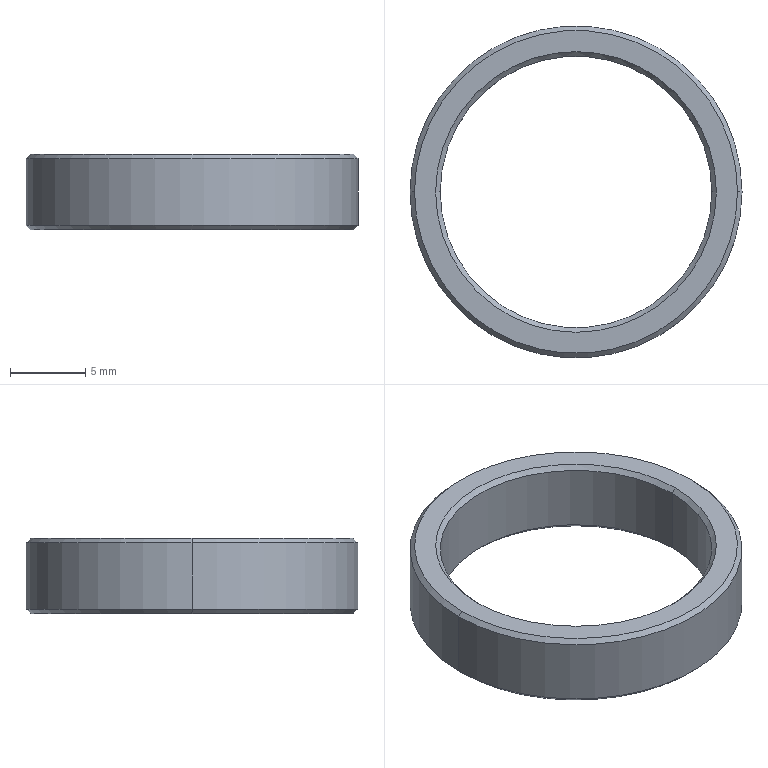Part | SolidWorks | features Chamfer 1, Extrusion 1, ICE 1 | 1 solid | 14 faces | box 22 x 22 x 5 mm | volume 617.009 mm3 | cone 8 | cylinder 4 | plane 2 | commonest cylinder face diameters 18 x2 22 x2
STEP:
#1=CARTESIAN_POINT('',(-9.,0.,4.7));
#2=VERTEX_POINT('',#1);
#3=CARTESIAN_POINT('',(9.,0.,4.7));
#4=VERTEX_POINT('',#3);
#5=CARTESIAN_POINT('',(0.,0.,4.7));
#6=DIRECTION('',(0.,0.,1.));
#7=DIRECTION('',(1.,0.,0.));
#8=AXIS2_PLACEMENT_3D('',#5,#6,#7);
#9=CIRCLE('',#8,9.);
#10=EDGE_CURVE('',#2,#4,#9,.T.);
#11=ORIENTED_EDGE('',*,*,#10,.F.);
#12=CARTESIAN_POINT('',(-9.3,0.,5.));
#13=VERTEX_POINT('',#12);
#14=CARTESIAN_POINT('',(-9.,0.,4.7));
#15=DIRECTION('',(-0.7071,0.,0.7071));
#16=VECTOR('',#15,1000.);
#17=LINE('',#14,#16);
#18=EDGE_CURVE('',#2,#13,#17,.T.);
#19=ORIENTED_EDGE('',*,*,#18,.T.);
#20=CARTESIAN_POINT('',(9.3,0.,5.));
#21=VERTEX_POINT('',#20);
#22=CARTESIAN_POINT('',(0.,0.,5.));
#23=DIRECTION('',(0.,0.,-1.));
#24=DIRECTION('',(1.,0.,0.));
#25=AXIS2_PLACEMENT_3D('',#22,#23,#24);
#26=CIRCLE('',#25,9.3);
#27=EDGE_CURVE('',#21,#13,#26,.T.);
#28=ORIENTED_EDGE('',*,*,#27,.F.);
#29=CARTESIAN_POINT('',(9.,0.,4.7));
#30=DIRECTION('',(0.7071,0.,0.7071));
#31=VECTOR('',#30,1000.);
#32=LINE('',#29,#31);
#33=EDGE_CURVE('',#4,#21,#32,.T.);
#34=ORIENTED_EDGE('',*,*,#33,.F.);
#35=EDGE_LOOP('',(#11,#19,#28,#34));
#36=FACE_OUTER_BOUND('',#35,.T.);
#37=CARTESIAN_POINT('',(0.,0.,4.7));
#38=DIRECTION('',(0.,0.,1.));
#39=DIRECTION('',(1.,0.,0.));
#40=AXIS2_PLACEMENT_3D('',#37,#38,#39);
#41=CONICAL_SURFACE('',#40,9.,0.7854);
#42=ADVANCED_FACE('',(#36),#41,.F.);
#43=CARTESIAN_POINT('',(9.,0.,0.3));
#44=VERTEX_POINT('',#43);
#45=CARTESIAN_POINT('',(-9.,0.,0.3));
#46=VERTEX_POINT('',#45);
#47=CARTESIAN_POINT('',(0.,0.,0.3));
#48=DIRECTION('',(0.,0.,-1.));
#49=DIRECTION('',(1.,0.,0.));
#50=AXIS2_PLACEMENT_3D('',#47,#48,#49);
#51=CIRCLE('',#50,9.);
#52=EDGE_CURVE('',#44,#46,#51,.T.);
#53=ORIENTED_EDGE('',*,*,#52,.F.);
#54=CARTESIAN_POINT('',(9.3,0.,0.));
#55=VERTEX_POINT('',#54);
#56=CARTESIAN_POINT('',(9.3,0.,0.));
#57=DIRECTION('',(0.7071,0.,-0.7071));
#58=VECTOR('',#57,1000.);
#59=LINE('',#56,#58);
#60=EDGE_CURVE('',#44,#55,#59,.T.);
#61=ORIENTED_EDGE('',*,*,#60,.T.);
#62=CARTESIAN_POINT('',(-9.3,0.,0.));
#63=VERTEX_POINT('',#62);
#64=CARTESIAN_POINT('',(0.,0.,0.));
#65=DIRECTION('',(0.,0.,1.));
#66=DIRECTION('',(1.,0.,0.));
#67=AXIS2_PLACEMENT_3D('',#64,#65,#66);
#68=CIRCLE('',#67,9.3);
#69=EDGE_CURVE('',#63,#55,#68,.T.);
#70=ORIENTED_EDGE('',*,*,#69,.F.);
#71=CARTESIAN_POINT('',(-9.3,0.,0.));
#72=DIRECTION('',(-0.7071,0.,-0.7071));
#73=VECTOR('',#72,1000.);
#74=LINE('',#71,#73);
#75=EDGE_CURVE('',#46,#63,#74,.T.);
#76=ORIENTED_EDGE('',*,*,#75,.F.);
#77=EDGE_LOOP('',(#53,#61,#70,#76));
#78=FACE_OUTER_BOUND('',#77,.T.);
#79=CARTESIAN_POINT('',(0.,0.,0.));
#80=DIRECTION('',(0.,0.,-1.));
#81=DIRECTION('',(-1.,0.,0.));
#82=AXIS2_PLACEMENT_3D('',#79,#80,#81);
#83=CONICAL_SURFACE('',#82,9.3,0.7854);
#84=ADVANCED_FACE('',(#78),#83,.F.);
#85=CARTESIAN_POINT('',(10.7,0.,5.));
#86=VERTEX_POINT('',#85);
#87=CARTESIAN_POINT('',(-10.7,0.,5.));
#88=VERTEX_POINT('',#87);
#89=CARTESIAN_POINT('',(0.,0.,5.));
#90=DIRECTION('',(0.,0.,1.));
#91=DIRECTION('',(1.,0.,0.));
#92=AXIS2_PLACEMENT_3D('',#89,#90,#91);
#93=CIRCLE('',#92,10.7);
#94=EDGE_CURVE('',#86,#88,#93,.T.);
#95=ORIENTED_EDGE('',*,*,#94,.F.);
#96=CARTESIAN_POINT('',(11.,0.,4.7));
#97=VERTEX_POINT('',#96);
#98=CARTESIAN_POINT('',(10.7,0.,5.));
#99=DIRECTION('',(0.7071,0.,-0.7071));
#100=VECTOR('',#99,1000.);
#101=LINE('',#98,#100);
#102=EDGE_CURVE('',#86,#97,#101,.T.);
#103=ORIENTED_EDGE('',*,*,#102,.T.);
#104=CARTESIAN_POINT('',(-11.,0.,4.7));
#105=VERTEX_POINT('',#104);
#106=CARTESIAN_POINT('',(0.,0.,4.7));
#107=DIRECTION('',(0.,0.,-1.));
#108=DIRECTION('',(1.,0.,0.));
#109=AXIS2_PLACEMENT_3D('',#106,#107,#108);
#110=CIRCLE('',#109,11.);
#111=EDGE_CURVE('',#105,#97,#110,.T.);
#112=ORIENTED_EDGE('',*,*,#111,.F.);
#113=CARTESIAN_POINT('',(-10.7,0.,5.));
#114=DIRECTION('',(-0.7071,0.,-0.7071));
#115=VECTOR('',#114,1000.);
#116=LINE('',#113,#115);
#117=EDGE_CURVE('',#88,#105,#116,.T.);
#118=ORIENTED_EDGE('',*,*,#117,.F.);
#119=EDGE_LOOP('',(#95,#103,#112,#118));
#120=FACE_OUTER_BOUND('',#119,.T.);
#121=CARTESIAN_POINT('',(0.,0.,5.));
#122=DIRECTION('',(0.,0.,-1.));
#123=DIRECTION('',(-1.,0.,0.));
#124=AXIS2_PLACEMENT_3D('',#121,#122,#123);
#125=CONICAL_SURFACE('',#124,10.7,0.7854);
#126=ADVANCED_FACE('',(#120),#125,.T.);
#127=CARTESIAN_POINT('',(-10.7,0.,0.));
#128=VERTEX_POINT('',#127);
#129=CARTESIAN_POINT('',(10.7,0.,0.));
#130=VERTEX_POINT('',#129);
#131=CARTESIAN_POINT('',(0.,0.,0.));
#132=DIRECTION('',(0.,0.,-1.));
#133=DIRECTION('',(1.,0.,0.));
#134=AXIS2_PLACEMENT_3D('',#131,#132,#133);
#135=CIRCLE('',#134,10.7);
#136=EDGE_CURVE('',#128,#130,#135,.T.);
#137=ORIENTED_EDGE('',*,*,#136,.F.);
#138=CARTESIAN_POINT('',(-11.,0.,0.3));
#139=VERTEX_POINT('',#138);
#140=CARTESIAN_POINT('',(-11.,0.,0.3));
#141=DIRECTION('',(-0.7071,0.,0.7071));
#142=VECTOR('',#141,1000.);
#143=LINE('',#140,#142);
#144=EDGE_CURVE('',#128,#139,#143,.T.);
#145=ORIENTED_EDGE('',*,*,#144,.T.);
#146=CARTESIAN_POINT('',(11.,0.,0.3));
#147=VERTEX_POINT('',#146);
#148=CARTESIAN_POINT('',(0.,0.,0.3));
#149=DIRECTION('',(0.,0.,1.));
#150=DIRECTION('',(1.,0.,0.));
#151=AXIS2_PLACEMENT_3D('',#148,#149,#150);
#152=CIRCLE('',#151,11.);
#153=EDGE_CURVE('',#147,#139,#152,.T.);
#154=ORIENTED_EDGE('',*,*,#153,.F.);
#155=CARTESIAN_POINT('',(11.,0.,0.3));
#156=DIRECTION('',(0.7071,0.,0.7071));
#157=VECTOR('',#156,1000.);
#158=LINE('',#155,#157);
#159=EDGE_CURVE('',#130,#147,#158,.T.);
#160=ORIENTED_EDGE('',*,*,#159,.F.);
#161=EDGE_LOOP('',(#137,#145,#154,#160));
#162=FACE_OUTER_BOUND('',#161,.T.);
#163=CARTESIAN_POINT('',(0.,0.,0.3));
#164=DIRECTION('',(0.,0.,1.));
#165=DIRECTION('',(1.,0.,0.));
#166=AXIS2_PLACEMENT_3D('',#163,#164,#165);
#167=CONICAL_SURFACE('',#166,11.,0.7854);
#168=ADVANCED_FACE('',(#162),#167,.T.);
#169=ORIENTED_EDGE('',*,*,#52,.T.);
#170=CARTESIAN_POINT('',(-9.,0.,0.));
#171=DIRECTION('',(0.,0.,1.));
#172=VECTOR('',#171,1000.);
#173=LINE('',#170,#172);
#174=EDGE_CURVE('',#46,#2,#173,.T.);
#175=ORIENTED_EDGE('',*,*,#174,.T.);
#176=ORIENTED_EDGE('',*,*,#10,.T.);
#177=CARTESIAN_POINT('',(9.,0.,0.));
#178=DIRECTION('',(0.,0.,1.));
#179=VECTOR('',#178,1000.);
#180=LINE('',#177,#179);
#181=EDGE_CURVE('',#44,#4,#180,.T.);
#182=ORIENTED_EDGE('',*,*,#181,.F.);
#183=EDGE_LOOP('',(#169,#175,#176,#182));
#184=FACE_OUTER_BOUND('',#183,.T.);
#185=CARTESIAN_POINT('',(0.,0.,0.));
#186=DIRECTION('',(0.,0.,1.));
#187=DIRECTION('',(1.,0.,0.));
#188=AXIS2_PLACEMENT_3D('',#185,#186,#187);
#189=CYLINDRICAL_SURFACE('',#188,9.);
#190=ADVANCED_FACE('',(#184),#189,.F.);
#191=ORIENTED_EDGE('',*,*,#111,.T.);
#192=CARTESIAN_POINT('',(11.,0.,5.));
#193=DIRECTION('',(0.,0.,-1.));
#194=VECTOR('',#193,1000.);
#195=LINE('',#192,#194);
#196=EDGE_CURVE('',#97,#147,#195,.T.);
#197=ORIENTED_EDGE('',*,*,#196,.T.);
#198=ORIENTED_EDGE('',*,*,#153,.T.);
#199=CARTESIAN_POINT('',(-11.,0.,5.));
#200=DIRECTION('',(0.,0.,-1.));
#201=VECTOR('',#200,1000.);
#202=LINE('',#199,#201);
#203=EDGE_CURVE('',#105,#139,#202,.T.);
#204=ORIENTED_EDGE('',*,*,#203,.F.);
#205=EDGE_LOOP('',(#191,#197,#198,#204));
#206=FACE_OUTER_BOUND('',#205,.T.);
#207=CARTESIAN_POINT('',(0.,0.,5.));
#208=DIRECTION('',(0.,0.,-1.));
#209=DIRECTION('',(-1.,0.,0.));
#210=AXIS2_PLACEMENT_3D('',#207,#208,#209);
#211=CYLINDRICAL_SURFACE('',#210,11.);
#212=ADVANCED_FACE('',(#206),#211,.T.);
#213=ORIENTED_EDGE('',*,*,#196,.F.);
#214=CARTESIAN_POINT('',(0.,0.,4.7));
#215=DIRECTION('',(0.,0.,-1.));
#216=DIRECTION('',(1.,0.,0.));
#217=AXIS2_PLACEMENT_3D('',#214,#215,#216);
#218=CIRCLE('',#217,11.);
#219=EDGE_CURVE('',#97,#105,#218,.T.);
#220=ORIENTED_EDGE('',*,*,#219,.T.);
#221=ORIENTED_EDGE('',*,*,#203,.T.);
#222=CARTESIAN_POINT('',(0.,0.,0.3));
#223=DIRECTION('',(0.,0.,1.));
#224=DIRECTION('',(1.,0.,0.));
#225=AXIS2_PLACEMENT_3D('',#222,#223,#224);
#226=CIRCLE('',#225,11.);
#227=EDGE_CURVE('',#139,#147,#226,.T.);
#228=ORIENTED_EDGE('',*,*,#227,.T.);
#229=EDGE_LOOP('',(#213,#220,#221,#228));
#230=FACE_OUTER_BOUND('',#229,.T.);
#231=CARTESIAN_POINT('',(0.,0.,5.));
#232=DIRECTION('',(0.,0.,-1.));
#233=DIRECTION('',(-1.,0.,0.));
#234=AXIS2_PLACEMENT_3D('',#231,#232,#233);
#235=CYLINDRICAL_SURFACE('',#234,11.);
#236=ADVANCED_FACE('',(#230),#235,.T.);
#237=CARTESIAN_POINT('',(0.,0.,5.));
#238=DIRECTION('',(0.,0.,1.));
#239=DIRECTION('',(1.,0.,0.));
#240=AXIS2_PLACEMENT_3D('',#237,#238,#239);
#241=CIRCLE('',#240,10.7);
#242=EDGE_CURVE('',#88,#86,#241,.T.);
#243=ORIENTED_EDGE('',*,*,#242,.T.);
#244=ORIENTED_EDGE('',*,*,#94,.T.);
#245=EDGE_LOOP('',(#243,#244));
#246=FACE_OUTER_BOUND('',#245,.T.);
#247=ORIENTED_EDGE('',*,*,#27,.T.);
#248=CARTESIAN_POINT('',(0.,0.,5.));
#249=DIRECTION('',(0.,0.,-1.));
#250=DIRECTION('',(1.,0.,0.));
#251=AXIS2_PLACEMENT_3D('',#248,#249,#250);
#252=CIRCLE('',#251,9.3);
#253=EDGE_CURVE('',#13,#21,#252,.T.);
#254=ORIENTED_EDGE('',*,*,#253,.T.);
#255=EDGE_LOOP('',(#247,#254));
#256=FACE_BOUND('',#255,.T.);
#257=CARTESIAN_POINT('',(0.,0.,5.));
#258=DIRECTION('',(0.,0.,1.));
#259=DIRECTION('',(1.,0.,0.));
#260=AXIS2_PLACEMENT_3D('',#257,#258,#259);
#261=PLANE('',#260);
#262=ADVANCED_FACE('',(#246,#256),#261,.T.);
#263=CARTESIAN_POINT('',(0.,0.,0.));
#264=DIRECTION('',(0.,0.,-1.));
#265=DIRECTION('',(1.,0.,0.));
#266=AXIS2_PLACEMENT_3D('',#263,#264,#265);
#267=CIRCLE('',#266,10.7);
#268=EDGE_CURVE('',#130,#128,#267,.T.);
#269=ORIENTED_EDGE('',*,*,#268,.T.);
#270=ORIENTED_EDGE('',*,*,#136,.T.);
#271=EDGE_LOOP('',(#269,#270));
#272=FACE_OUTER_BOUND('',#271,.T.);
#273=ORIENTED_EDGE('',*,*,#69,.T.);
#274=CARTESIAN_POINT('',(0.,0.,0.));
#275=DIRECTION('',(0.,0.,1.));
#276=DIRECTION('',(1.,0.,0.));
#277=AXIS2_PLACEMENT_3D('',#274,#275,#276);
#278=CIRCLE('',#277,9.3);
#279=EDGE_CURVE('',#55,#63,#278,.T.);
#280=ORIENTED_EDGE('',*,*,#279,.T.);
#281=EDGE_LOOP('',(#273,#280));
#282=FACE_BOUND('',#281,.T.);
#283=CARTESIAN_POINT('',(0.,0.,0.));
#284=DIRECTION('',(0.,0.,1.));
#285=DIRECTION('',(1.,0.,0.));
#286=AXIS2_PLACEMENT_3D('',#283,#284,#285);
#287=PLANE('',#286);
#288=ADVANCED_FACE('',(#272,#282),#287,.F.);
#289=ORIENTED_EDGE('',*,*,#174,.F.);
#290=CARTESIAN_POINT('',(0.,0.,0.3));
#291=DIRECTION('',(0.,0.,-1.));
#292=DIRECTION('',(1.,0.,0.));
#293=AXIS2_PLACEMENT_3D('',#290,#291,#292);
#294=CIRCLE('',#293,9.);
#295=EDGE_CURVE('',#46,#44,#294,.T.);
#296=ORIENTED_EDGE('',*,*,#295,.T.);
#297=ORIENTED_EDGE('',*,*,#181,.T.);
#298=CARTESIAN_POINT('',(0.,0.,4.7));
#299=DIRECTION('',(0.,0.,1.));
#300=DIRECTION('',(1.,0.,0.));
#301=AXIS2_PLACEMENT_3D('',#298,#299,#300);
#302=CIRCLE('',#301,9.);
#303=EDGE_CURVE('',#4,#2,#302,.T.);
#304=ORIENTED_EDGE('',*,*,#303,.T.);
#305=EDGE_LOOP('',(#289,#296,#297,#304));
#306=FACE_OUTER_BOUND('',#305,.T.);
#307=CARTESIAN_POINT('',(0.,0.,0.));
#308=DIRECTION('',(0.,0.,1.));
#309=DIRECTION('',(1.,0.,0.));
#310=AXIS2_PLACEMENT_3D('',#307,#308,#309);
#311=CYLINDRICAL_SURFACE('',#310,9.);
#312=ADVANCED_FACE('',(#306),#311,.F.);
#313=ORIENTED_EDGE('',*,*,#144,.F.);
#314=ORIENTED_EDGE('',*,*,#268,.F.);
#315=ORIENTED_EDGE('',*,*,#159,.T.);
#316=ORIENTED_EDGE('',*,*,#227,.F.);
#317=EDGE_LOOP('',(#313,#314,#315,#316));
#318=FACE_OUTER_BOUND('',#317,.T.);
#319=CARTESIAN_POINT('',(0.,0.,0.3));
#320=DIRECTION('',(0.,0.,1.));
#321=DIRECTION('',(1.,0.,0.));
#322=AXIS2_PLACEMENT_3D('',#319,#320,#321);
#323=CONICAL_SURFACE('',#322,11.,0.7854);
#324=ADVANCED_FACE('',(#318),#323,.T.);
#325=ORIENTED_EDGE('',*,*,#102,.F.);
#326=ORIENTED_EDGE('',*,*,#242,.F.);
#327=ORIENTED_EDGE('',*,*,#117,.T.);
#328=ORIENTED_EDGE('',*,*,#219,.F.);
#329=EDGE_LOOP('',(#325,#326,#327,#328));
#330=FACE_OUTER_BOUND('',#329,.T.);
#331=CARTESIAN_POINT('',(0.,0.,5.));
#332=DIRECTION('',(0.,0.,-1.));
#333=DIRECTION('',(-1.,0.,0.));
#334=AXIS2_PLACEMENT_3D('',#331,#332,#333);
#335=CONICAL_SURFACE('',#334,10.7,0.7854);
#336=ADVANCED_FACE('',(#330),#335,.T.);
#337=ORIENTED_EDGE('',*,*,#60,.F.);
#338=ORIENTED_EDGE('',*,*,#295,.F.);
#339=ORIENTED_EDGE('',*,*,#75,.T.);
#340=ORIENTED_EDGE('',*,*,#279,.F.);
#341=EDGE_LOOP('',(#337,#338,#339,#340));
#342=FACE_OUTER_BOUND('',#341,.T.);
#343=CARTESIAN_POINT('',(0.,0.,0.));
#344=DIRECTION('',(0.,0.,-1.));
#345=DIRECTION('',(-1.,0.,0.));
#346=AXIS2_PLACEMENT_3D('',#343,#344,#345);
#347=CONICAL_SURFACE('',#346,9.3,0.7854);
#348=ADVANCED_FACE('',(#342),#347,.F.);
#349=ORIENTED_EDGE('',*,*,#18,.F.);
#350=ORIENTED_EDGE('',*,*,#303,.F.);
#351=ORIENTED_EDGE('',*,*,#33,.T.);
#352=ORIENTED_EDGE('',*,*,#253,.F.);
#353=EDGE_LOOP('',(#349,#350,#351,#352));
#354=FACE_OUTER_BOUND('',#353,.T.);
#355=CARTESIAN_POINT('',(0.,0.,4.7));
#356=DIRECTION('',(0.,0.,1.));
#357=DIRECTION('',(1.,0.,0.));
#358=AXIS2_PLACEMENT_3D('',#355,#356,#357);
#359=CONICAL_SURFACE('',#358,9.,0.7854);
#360=ADVANCED_FACE('',(#354),#359,.F.);
#361=CLOSED_SHELL('',(#42,#84,#126,#168,#190,#212,#236,#262,#288,#312,#324,#336,#348,#360));
#362=MANIFOLD_SOLID_BREP('',#361);
#363=CARTESIAN_POINT('',(0.,0.,0.));
#364=DIRECTION('',(0.,0.,1.));
#365=DIRECTION('',(1.,0.,0.));
#366=AXIS2_PLACEMENT_3D('',#363,#364,#365);
#367=(LENGTH_UNIT()NAMED_UNIT(*)SI_UNIT(.MILLI.,.METRE.));
#368=UNCERTAINTY_MEASURE_WITH_UNIT(LENGTH_MEASURE(0.00001),#367,'','');
#369=(NAMED_UNIT(*)PLANE_ANGLE_UNIT()SI_UNIT($,.RADIAN.));
#370=(NAMED_UNIT(*)SI_UNIT($,.STERADIAN.)SOLID_ANGLE_UNIT());
#371=(GEOMETRIC_REPRESENTATION_CONTEXT(3)GLOBAL_UNCERTAINTY_ASSIGNED_CONTEXT((#368))GLOBAL_UNIT_ASSIGNED_CONTEXT((#367,#369,#370))REPRESENTATION_CONTEXT('',''));
#372=ADVANCED_BREP_SHAPE_REPRESENTATION('',(#362,#366),#371);